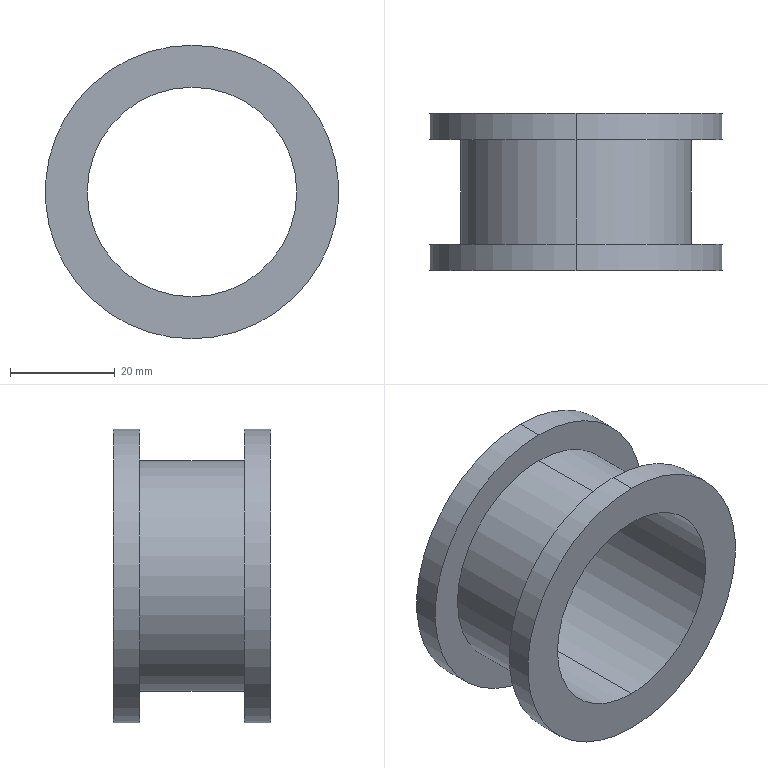Part | STEP file | outer coil1 | 1 solid | 12 faces | box 56 x 30 x 56 mm | volume 17342 mm3 | cylinder 8 | plane 4 | commonest cylinder face diameters 56 x4 40 x2 44 x2
STEP:
#1=CARTESIAN_POINT('',(0.,-10.,22.));
#2=VERTEX_POINT('',#1);
#3=CARTESIAN_POINT('',(0.,-10.,-22.));
#4=VERTEX_POINT('',#3);
#5=CARTESIAN_POINT('',(0.,-10.,0.));
#6=DIRECTION('',(0.,1.,0.));
#7=DIRECTION('',(0.,0.,1.));
#8=AXIS2_PLACEMENT_3D('',#5,#6,#7);
#9=CIRCLE('',#8,22.);
#10=EDGE_CURVE('',#2,#4,#9,.T.);
#11=ORIENTED_EDGE('',*,*,#10,.T.);
#12=CARTESIAN_POINT('',(0.,10.,-22.));
#13=VERTEX_POINT('',#12);
#14=CARTESIAN_POINT('',(0.,13.555,-22.));
#15=DIRECTION('',(0.,1.,0.));
#16=VECTOR('',#15,1000.);
#17=LINE('',#14,#16);
#18=EDGE_CURVE('',#4,#13,#17,.T.);
#19=ORIENTED_EDGE('',*,*,#18,.T.);
#20=CARTESIAN_POINT('',(0.,10.,22.));
#21=VERTEX_POINT('',#20);
#22=CARTESIAN_POINT('',(0.,10.,0.));
#23=DIRECTION('',(0.,1.,0.));
#24=DIRECTION('',(0.,0.,1.));
#25=AXIS2_PLACEMENT_3D('',#22,#23,#24);
#26=CIRCLE('',#25,22.);
#27=EDGE_CURVE('',#21,#13,#26,.T.);
#28=ORIENTED_EDGE('',*,*,#27,.F.);
#29=CARTESIAN_POINT('',(0.,13.555,22.));
#30=DIRECTION('',(0.,1.,0.));
#31=VECTOR('',#30,1000.);
#32=LINE('',#29,#31);
#33=EDGE_CURVE('',#2,#21,#32,.T.);
#34=ORIENTED_EDGE('',*,*,#33,.F.);
#35=EDGE_LOOP('',(#11,#19,#28,#34));
#36=FACE_OUTER_BOUND('',#35,.T.);
#37=CARTESIAN_POINT('',(0.,13.555,0.));
#38=DIRECTION('',(0.,1.,0.));
#39=DIRECTION('',(0.,0.,1.));
#40=AXIS2_PLACEMENT_3D('',#37,#38,#39);
#41=CYLINDRICAL_SURFACE('',#40,22.);
#42=ADVANCED_FACE('',(#36),#41,.T.);
#43=CARTESIAN_POINT('',(0.,-15.,-20.));
#44=VERTEX_POINT('',#43);
#45=CARTESIAN_POINT('',(0.,-15.,20.));
#46=VERTEX_POINT('',#45);
#47=CARTESIAN_POINT('',(0.,-15.,0.));
#48=DIRECTION('',(0.,1.,0.));
#49=DIRECTION('',(0.,0.,1.));
#50=AXIS2_PLACEMENT_3D('',#47,#48,#49);
#51=CIRCLE('',#50,20.);
#52=EDGE_CURVE('',#44,#46,#51,.T.);
#53=ORIENTED_EDGE('',*,*,#52,.F.);
#54=CARTESIAN_POINT('',(0.,15.,-20.));
#55=VERTEX_POINT('',#54);
#56=CARTESIAN_POINT('',(0.,65.771,-20.));
#57=DIRECTION('',(0.,1.,0.));
#58=VECTOR('',#57,1000.);
#59=LINE('',#56,#58);
#60=EDGE_CURVE('',#44,#55,#59,.T.);
#61=ORIENTED_EDGE('',*,*,#60,.T.);
#62=CARTESIAN_POINT('',(0.,15.,20.));
#63=VERTEX_POINT('',#62);
#64=CARTESIAN_POINT('',(0.,15.,0.));
#65=DIRECTION('',(0.,1.,0.));
#66=DIRECTION('',(0.,0.,1.));
#67=AXIS2_PLACEMENT_3D('',#64,#65,#66);
#68=CIRCLE('',#67,20.);
#69=EDGE_CURVE('',#55,#63,#68,.T.);
#70=ORIENTED_EDGE('',*,*,#69,.T.);
#71=CARTESIAN_POINT('',(0.,65.771,20.));
#72=DIRECTION('',(0.,1.,0.));
#73=VECTOR('',#72,1000.);
#74=LINE('',#71,#73);
#75=EDGE_CURVE('',#46,#63,#74,.T.);
#76=ORIENTED_EDGE('',*,*,#75,.F.);
#77=EDGE_LOOP('',(#53,#61,#70,#76));
#78=FACE_OUTER_BOUND('',#77,.T.);
#79=CARTESIAN_POINT('',(0.,65.771,0.));
#80=DIRECTION('',(0.,1.,0.));
#81=DIRECTION('',(0.,0.,1.));
#82=AXIS2_PLACEMENT_3D('',#79,#80,#81);
#83=CYLINDRICAL_SURFACE('',#82,20.);
#84=ADVANCED_FACE('',(#78),#83,.F.);
#85=CARTESIAN_POINT('',(0.,10.,28.));
#86=VERTEX_POINT('',#85);
#87=CARTESIAN_POINT('',(0.,10.,-28.));
#88=VERTEX_POINT('',#87);
#89=CARTESIAN_POINT('',(0.,10.,0.));
#90=DIRECTION('',(0.,1.,0.));
#91=DIRECTION('',(0.,0.,1.));
#92=AXIS2_PLACEMENT_3D('',#89,#90,#91);
#93=CIRCLE('',#92,28.);
#94=EDGE_CURVE('',#86,#88,#93,.T.);
#95=ORIENTED_EDGE('',*,*,#94,.T.);
#96=CARTESIAN_POINT('',(0.,15.,-28.));
#97=VERTEX_POINT('',#96);
#98=CARTESIAN_POINT('',(0.,65.771,-28.));
#99=DIRECTION('',(0.,1.,0.));
#100=VECTOR('',#99,1000.);
#101=LINE('',#98,#100);
#102=EDGE_CURVE('',#88,#97,#101,.T.);
#103=ORIENTED_EDGE('',*,*,#102,.T.);
#104=CARTESIAN_POINT('',(0.,15.,28.));
#105=VERTEX_POINT('',#104);
#106=CARTESIAN_POINT('',(0.,15.,0.));
#107=DIRECTION('',(0.,1.,0.));
#108=DIRECTION('',(0.,0.,1.));
#109=AXIS2_PLACEMENT_3D('',#106,#107,#108);
#110=CIRCLE('',#109,28.);
#111=EDGE_CURVE('',#105,#97,#110,.T.);
#112=ORIENTED_EDGE('',*,*,#111,.F.);
#113=CARTESIAN_POINT('',(0.,65.771,28.));
#114=DIRECTION('',(0.,1.,0.));
#115=VECTOR('',#114,1000.);
#116=LINE('',#113,#115);
#117=EDGE_CURVE('',#86,#105,#116,.T.);
#118=ORIENTED_EDGE('',*,*,#117,.F.);
#119=EDGE_LOOP('',(#95,#103,#112,#118));
#120=FACE_OUTER_BOUND('',#119,.T.);
#121=CARTESIAN_POINT('',(0.,65.771,0.));
#122=DIRECTION('',(0.,1.,0.));
#123=DIRECTION('',(0.,0.,1.));
#124=AXIS2_PLACEMENT_3D('',#121,#122,#123);
#125=CYLINDRICAL_SURFACE('',#124,28.);
#126=ADVANCED_FACE('',(#120),#125,.T.);
#127=CARTESIAN_POINT('',(0.,-15.,28.));
#128=VERTEX_POINT('',#127);
#129=CARTESIAN_POINT('',(0.,-15.,-28.));
#130=VERTEX_POINT('',#129);
#131=CARTESIAN_POINT('',(0.,-15.,0.));
#132=DIRECTION('',(0.,1.,0.));
#133=DIRECTION('',(0.,0.,1.));
#134=AXIS2_PLACEMENT_3D('',#131,#132,#133);
#135=CIRCLE('',#134,28.);
#136=EDGE_CURVE('',#128,#130,#135,.T.);
#137=ORIENTED_EDGE('',*,*,#136,.T.);
#138=CARTESIAN_POINT('',(0.,-10.,-28.));
#139=VERTEX_POINT('',#138);
#140=CARTESIAN_POINT('',(0.,65.771,-28.));
#141=DIRECTION('',(0.,1.,0.));
#142=VECTOR('',#141,1000.);
#143=LINE('',#140,#142);
#144=EDGE_CURVE('',#130,#139,#143,.T.);
#145=ORIENTED_EDGE('',*,*,#144,.T.);
#146=CARTESIAN_POINT('',(0.,-10.,28.));
#147=VERTEX_POINT('',#146);
#148=CARTESIAN_POINT('',(0.,-10.,0.));
#149=DIRECTION('',(0.,1.,0.));
#150=DIRECTION('',(0.,0.,1.));
#151=AXIS2_PLACEMENT_3D('',#148,#149,#150);
#152=CIRCLE('',#151,28.);
#153=EDGE_CURVE('',#147,#139,#152,.T.);
#154=ORIENTED_EDGE('',*,*,#153,.F.);
#155=CARTESIAN_POINT('',(0.,65.771,28.));
#156=DIRECTION('',(0.,1.,0.));
#157=VECTOR('',#156,1000.);
#158=LINE('',#155,#157);
#159=EDGE_CURVE('',#128,#147,#158,.T.);
#160=ORIENTED_EDGE('',*,*,#159,.F.);
#161=EDGE_LOOP('',(#137,#145,#154,#160));
#162=FACE_OUTER_BOUND('',#161,.T.);
#163=CARTESIAN_POINT('',(0.,65.771,0.));
#164=DIRECTION('',(0.,1.,0.));
#165=DIRECTION('',(0.,0.,1.));
#166=AXIS2_PLACEMENT_3D('',#163,#164,#165);
#167=CYLINDRICAL_SURFACE('',#166,28.);
#168=ADVANCED_FACE('',(#162),#167,.T.);
#169=ORIENTED_EDGE('',*,*,#144,.F.);
#170=CARTESIAN_POINT('',(0.,-15.,0.));
#171=DIRECTION('',(0.,1.,0.));
#172=DIRECTION('',(0.,0.,1.));
#173=AXIS2_PLACEMENT_3D('',#170,#171,#172);
#174=CIRCLE('',#173,28.);
#175=EDGE_CURVE('',#130,#128,#174,.T.);
#176=ORIENTED_EDGE('',*,*,#175,.T.);
#177=ORIENTED_EDGE('',*,*,#159,.T.);
#178=CARTESIAN_POINT('',(0.,-10.,0.));
#179=DIRECTION('',(0.,1.,0.));
#180=DIRECTION('',(0.,0.,1.));
#181=AXIS2_PLACEMENT_3D('',#178,#179,#180);
#182=CIRCLE('',#181,28.);
#183=EDGE_CURVE('',#139,#147,#182,.T.);
#184=ORIENTED_EDGE('',*,*,#183,.F.);
#185=EDGE_LOOP('',(#169,#176,#177,#184));
#186=FACE_OUTER_BOUND('',#185,.T.);
#187=CARTESIAN_POINT('',(0.,65.771,0.));
#188=DIRECTION('',(0.,1.,0.));
#189=DIRECTION('',(0.,0.,1.));
#190=AXIS2_PLACEMENT_3D('',#187,#188,#189);
#191=CYLINDRICAL_SURFACE('',#190,28.);
#192=ADVANCED_FACE('',(#186),#191,.T.);
#193=ORIENTED_EDGE('',*,*,#102,.F.);
#194=CARTESIAN_POINT('',(0.,10.,0.));
#195=DIRECTION('',(0.,1.,0.));
#196=DIRECTION('',(0.,0.,1.));
#197=AXIS2_PLACEMENT_3D('',#194,#195,#196);
#198=CIRCLE('',#197,28.);
#199=EDGE_CURVE('',#88,#86,#198,.T.);
#200=ORIENTED_EDGE('',*,*,#199,.T.);
#201=ORIENTED_EDGE('',*,*,#117,.T.);
#202=CARTESIAN_POINT('',(0.,15.,0.));
#203=DIRECTION('',(0.,1.,0.));
#204=DIRECTION('',(0.,0.,1.));
#205=AXIS2_PLACEMENT_3D('',#202,#203,#204);
#206=CIRCLE('',#205,28.);
#207=EDGE_CURVE('',#97,#105,#206,.T.);
#208=ORIENTED_EDGE('',*,*,#207,.F.);
#209=EDGE_LOOP('',(#193,#200,#201,#208));
#210=FACE_OUTER_BOUND('',#209,.T.);
#211=CARTESIAN_POINT('',(0.,65.771,0.));
#212=DIRECTION('',(0.,1.,0.));
#213=DIRECTION('',(0.,0.,1.));
#214=AXIS2_PLACEMENT_3D('',#211,#212,#213);
#215=CYLINDRICAL_SURFACE('',#214,28.);
#216=ADVANCED_FACE('',(#210),#215,.T.);
#217=ORIENTED_EDGE('',*,*,#111,.T.);
#218=ORIENTED_EDGE('',*,*,#207,.T.);
#219=EDGE_LOOP('',(#217,#218));
#220=FACE_OUTER_BOUND('',#219,.T.);
#221=CARTESIAN_POINT('',(0.,15.,0.));
#222=DIRECTION('',(0.,1.,0.));
#223=DIRECTION('',(0.,0.,1.));
#224=AXIS2_PLACEMENT_3D('',#221,#222,#223);
#225=CIRCLE('',#224,20.);
#226=EDGE_CURVE('',#63,#55,#225,.T.);
#227=ORIENTED_EDGE('',*,*,#226,.F.);
#228=ORIENTED_EDGE('',*,*,#69,.F.);
#229=EDGE_LOOP('',(#227,#228));
#230=FACE_BOUND('',#229,.T.);
#231=CARTESIAN_POINT('',(-20.,15.,0.));
#232=DIRECTION('',(0.,1.,0.));
#233=DIRECTION('',(0.,0.,1.));
#234=AXIS2_PLACEMENT_3D('',#231,#232,#233);
#235=PLANE('',#234);
#236=ADVANCED_FACE('',(#220,#230),#235,.T.);
#237=ORIENTED_EDGE('',*,*,#60,.F.);
#238=CARTESIAN_POINT('',(0.,-15.,0.));
#239=DIRECTION('',(0.,1.,0.));
#240=DIRECTION('',(0.,0.,1.));
#241=AXIS2_PLACEMENT_3D('',#238,#239,#240);
#242=CIRCLE('',#241,20.);
#243=EDGE_CURVE('',#46,#44,#242,.T.);
#244=ORIENTED_EDGE('',*,*,#243,.F.);
#245=ORIENTED_EDGE('',*,*,#75,.T.);
#246=ORIENTED_EDGE('',*,*,#226,.T.);
#247=EDGE_LOOP('',(#237,#244,#245,#246));
#248=FACE_OUTER_BOUND('',#247,.T.);
#249=CARTESIAN_POINT('',(0.,65.771,0.));
#250=DIRECTION('',(0.,1.,0.));
#251=DIRECTION('',(0.,0.,1.));
#252=AXIS2_PLACEMENT_3D('',#249,#250,#251);
#253=CYLINDRICAL_SURFACE('',#252,20.);
#254=ADVANCED_FACE('',(#248),#253,.F.);
#255=ORIENTED_EDGE('',*,*,#243,.T.);
#256=ORIENTED_EDGE('',*,*,#52,.T.);
#257=EDGE_LOOP('',(#255,#256));
#258=FACE_BOUND('',#257,.T.);
#259=ORIENTED_EDGE('',*,*,#136,.F.);
#260=ORIENTED_EDGE('',*,*,#175,.F.);
#261=EDGE_LOOP('',(#259,#260));
#262=FACE_OUTER_BOUND('',#261,.T.);
#263=CARTESIAN_POINT('',(-20.,-15.,0.));
#264=DIRECTION('',(0.,-1.,0.));
#265=DIRECTION('',(0.,0.,-1.));
#266=AXIS2_PLACEMENT_3D('',#263,#264,#265);
#267=PLANE('',#266);
#268=ADVANCED_FACE('',(#258,#262),#267,.T.);
#269=ORIENTED_EDGE('',*,*,#10,.F.);
#270=CARTESIAN_POINT('',(0.,-10.,0.));
#271=DIRECTION('',(0.,1.,0.));
#272=DIRECTION('',(0.,0.,1.));
#273=AXIS2_PLACEMENT_3D('',#270,#271,#272);
#274=CIRCLE('',#273,22.);
#275=EDGE_CURVE('',#4,#2,#274,.T.);
#276=ORIENTED_EDGE('',*,*,#275,.F.);
#277=EDGE_LOOP('',(#269,#276));
#278=FACE_BOUND('',#277,.T.);
#279=ORIENTED_EDGE('',*,*,#153,.T.);
#280=ORIENTED_EDGE('',*,*,#183,.T.);
#281=EDGE_LOOP('',(#279,#280));
#282=FACE_OUTER_BOUND('',#281,.T.);
#283=CARTESIAN_POINT('',(-22.,-10.,0.));
#284=DIRECTION('',(0.,-1.,0.));
#285=DIRECTION('',(0.,0.,-1.));
#286=AXIS2_PLACEMENT_3D('',#283,#284,#285);
#287=PLANE('',#286);
#288=ADVANCED_FACE('',(#278,#282),#287,.F.);
#289=ORIENTED_EDGE('',*,*,#18,.F.);
#290=ORIENTED_EDGE('',*,*,#275,.T.);
#291=ORIENTED_EDGE('',*,*,#33,.T.);
#292=CARTESIAN_POINT('',(0.,10.,0.));
#293=DIRECTION('',(0.,1.,0.));
#294=DIRECTION('',(0.,0.,1.));
#295=AXIS2_PLACEMENT_3D('',#292,#293,#294);
#296=CIRCLE('',#295,22.);
#297=EDGE_CURVE('',#13,#21,#296,.T.);
#298=ORIENTED_EDGE('',*,*,#297,.F.);
#299=EDGE_LOOP('',(#289,#290,#291,#298));
#300=FACE_OUTER_BOUND('',#299,.T.);
#301=CARTESIAN_POINT('',(0.,13.555,0.));
#302=DIRECTION('',(0.,1.,0.));
#303=DIRECTION('',(0.,0.,1.));
#304=AXIS2_PLACEMENT_3D('',#301,#302,#303);
#305=CYLINDRICAL_SURFACE('',#304,22.);
#306=ADVANCED_FACE('',(#300),#305,.T.);
#307=ORIENTED_EDGE('',*,*,#94,.F.);
#308=ORIENTED_EDGE('',*,*,#199,.F.);
#309=EDGE_LOOP('',(#307,#308));
#310=FACE_OUTER_BOUND('',#309,.T.);
#311=ORIENTED_EDGE('',*,*,#27,.T.);
#312=ORIENTED_EDGE('',*,*,#297,.T.);
#313=EDGE_LOOP('',(#311,#312));
#314=FACE_BOUND('',#313,.T.);
#315=CARTESIAN_POINT('',(-22.,10.,0.));
#316=DIRECTION('',(0.,1.,0.));
#317=DIRECTION('',(0.,0.,1.));
#318=AXIS2_PLACEMENT_3D('',#315,#316,#317);
#319=PLANE('',#318);
#320=ADVANCED_FACE('',(#310,#314),#319,.F.);
#321=CLOSED_SHELL('',(#42,#84,#126,#168,#192,#216,#236,#254,#268,#288,#306,#320));
#322=MANIFOLD_SOLID_BREP('',#321);
#323=CARTESIAN_POINT('',(0.,0.,0.));
#324=DIRECTION('',(0.,0.,1.));
#325=DIRECTION('',(1.,0.,0.));
#326=AXIS2_PLACEMENT_3D('',#323,#324,#325);
#327=(LENGTH_UNIT()NAMED_UNIT(*)SI_UNIT(.MILLI.,.METRE.));
#328=UNCERTAINTY_MEASURE_WITH_UNIT(LENGTH_MEASURE(0.00001),#327,'','');
#329=(NAMED_UNIT(*)PLANE_ANGLE_UNIT()SI_UNIT($,.RADIAN.));
#330=(NAMED_UNIT(*)SI_UNIT($,.STERADIAN.)SOLID_ANGLE_UNIT());
#331=(GEOMETRIC_REPRESENTATION_CONTEXT(3)GLOBAL_UNCERTAINTY_ASSIGNED_CONTEXT((#328))GLOBAL_UNIT_ASSIGNED_CONTEXT((#327,#329,#330))REPRESENTATION_CONTEXT('',''));
#332=ADVANCED_BREP_SHAPE_REPRESENTATION('',(#322,#326),#331);